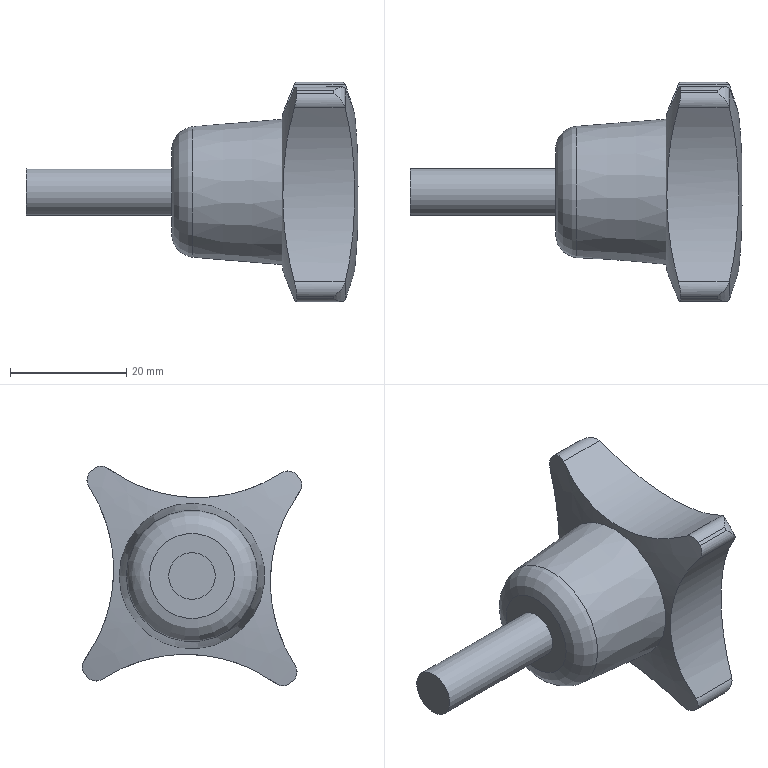Part | STEP file | 13468 | 1 solid | 27 faces | box 57.035 x 37.729 x 37.729 mm | volume 20662 mm3 | cylinder 17 | torus 5 | plane 2 | spline 2 | cone 1 | commonest cylinder face diameters 4 x8 50 x4 53 x4 8 x1